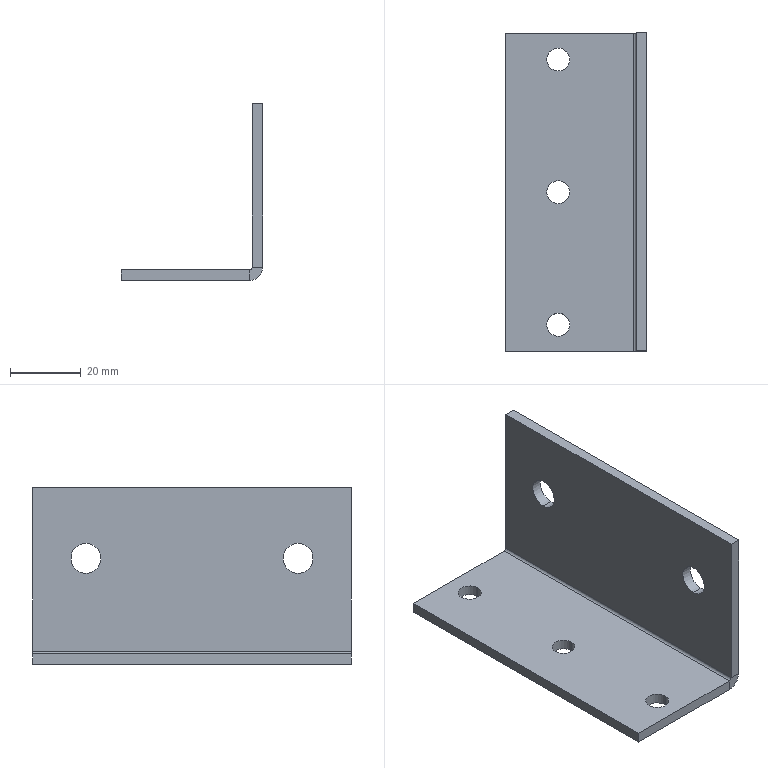Part | STEP file | PN_0001 connector code | 1 solid | 24 faces | box 40 x 90 x 50 mm | volume 22592 mm3 | cylinder 12 | plane 12 | commonest cylinder face diameters 6.5 x6 8.5 x4 1.473 x1 7.473 x1